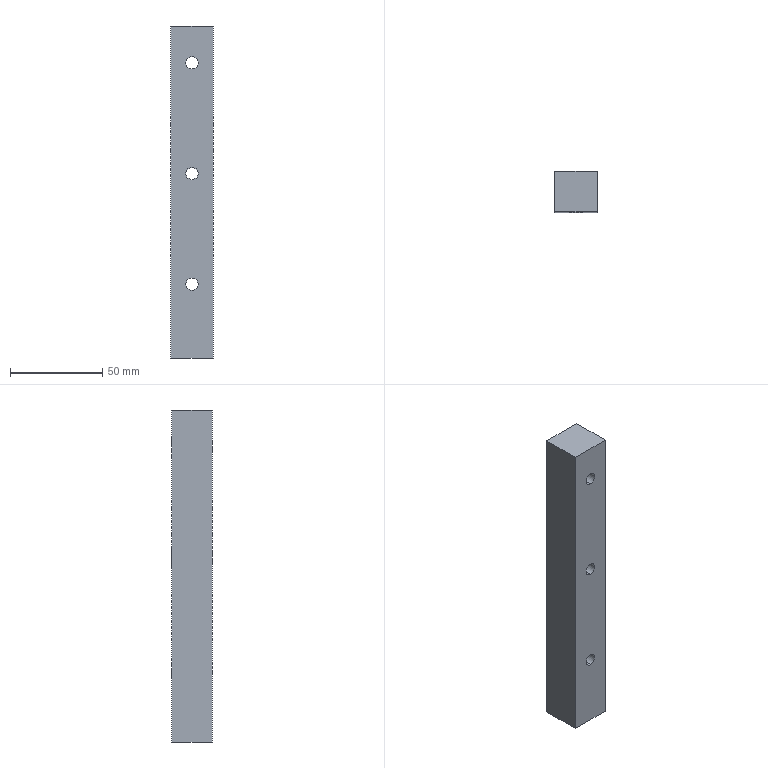Part | SolidWorks | features Extrusion 1, HoleWzd 1, LPattern 1 | 1 solid | 21 faces | box 23 x 22 x 180 mm | volume 87654 mm3 | cylinder 12 | plane 9 | commonest cylinder face diameters 6.6 x6 11 x6
STEP:
#1=CARTESIAN_POINT('',(11.5,15.6,34.5));
#2=VERTEX_POINT('',#1);
#3=CARTESIAN_POINT('',(11.5,15.6,45.5));
#4=VERTEX_POINT('',#3);
#5=CARTESIAN_POINT('',(11.5,15.6,40.));
#6=DIRECTION('',(0.,1.,0.));
#7=DIRECTION('',(0.,0.,1.));
#8=AXIS2_PLACEMENT_3D('',#5,#6,#7);
#9=CIRCLE('',#8,5.5);
#10=EDGE_CURVE('',#2,#4,#9,.T.);
#11=ORIENTED_EDGE('',*,*,#10,.F.);
#12=CARTESIAN_POINT('',(11.5,22.,34.5));
#13=VERTEX_POINT('',#12);
#14=CARTESIAN_POINT('',(11.5,22.,34.5));
#15=DIRECTION('',(0.,1.,0.));
#16=VECTOR('',#15,1000.);
#17=LINE('',#14,#16);
#18=EDGE_CURVE('',#2,#13,#17,.T.);
#19=ORIENTED_EDGE('',*,*,#18,.T.);
#20=CARTESIAN_POINT('',(11.5,22.,45.5));
#21=VERTEX_POINT('',#20);
#22=CARTESIAN_POINT('',(11.5,22.,40.));
#23=DIRECTION('',(0.,1.,0.));
#24=DIRECTION('',(0.,0.,1.));
#25=AXIS2_PLACEMENT_3D('',#22,#23,#24);
#26=CIRCLE('',#25,5.5);
#27=EDGE_CURVE('',#13,#21,#26,.T.);
#28=ORIENTED_EDGE('',*,*,#27,.T.);
#29=CARTESIAN_POINT('',(11.5,22.,45.5));
#30=DIRECTION('',(0.,1.,0.));
#31=VECTOR('',#30,1000.);
#32=LINE('',#29,#31);
#33=EDGE_CURVE('',#4,#21,#32,.T.);
#34=ORIENTED_EDGE('',*,*,#33,.F.);
#35=EDGE_LOOP('',(#11,#19,#28,#34));
#36=FACE_OUTER_BOUND('',#35,.T.);
#37=CARTESIAN_POINT('',(11.5,22.,40.));
#38=DIRECTION('',(0.,1.,0.));
#39=DIRECTION('',(0.,0.,1.));
#40=AXIS2_PLACEMENT_3D('',#37,#38,#39);
#41=CYLINDRICAL_SURFACE('',#40,5.5);
#42=ADVANCED_FACE('',(#36),#41,.F.);
#43=CARTESIAN_POINT('',(11.5,0.,36.7));
#44=VERTEX_POINT('',#43);
#45=CARTESIAN_POINT('',(11.5,0.,43.3));
#46=VERTEX_POINT('',#45);
#47=CARTESIAN_POINT('',(11.5,0.,40.));
#48=DIRECTION('',(0.,1.,0.));
#49=DIRECTION('',(0.,0.,1.));
#50=AXIS2_PLACEMENT_3D('',#47,#48,#49);
#51=CIRCLE('',#50,3.3);
#52=EDGE_CURVE('',#44,#46,#51,.T.);
#53=ORIENTED_EDGE('',*,*,#52,.F.);
#54=CARTESIAN_POINT('',(11.5,15.6,36.7));
#55=VERTEX_POINT('',#54);
#56=CARTESIAN_POINT('',(11.5,22.,36.7));
#57=DIRECTION('',(0.,1.,0.));
#58=VECTOR('',#57,1000.);
#59=LINE('',#56,#58);
#60=EDGE_CURVE('',#44,#55,#59,.T.);
#61=ORIENTED_EDGE('',*,*,#60,.T.);
#62=CARTESIAN_POINT('',(11.5,15.6,43.3));
#63=VERTEX_POINT('',#62);
#64=CARTESIAN_POINT('',(11.5,15.6,40.));
#65=DIRECTION('',(0.,1.,0.));
#66=DIRECTION('',(0.,0.,1.));
#67=AXIS2_PLACEMENT_3D('',#64,#65,#66);
#68=CIRCLE('',#67,3.3);
#69=EDGE_CURVE('',#55,#63,#68,.T.);
#70=ORIENTED_EDGE('',*,*,#69,.T.);
#71=CARTESIAN_POINT('',(11.5,22.,43.3));
#72=DIRECTION('',(0.,1.,0.));
#73=VECTOR('',#72,1000.);
#74=LINE('',#71,#73);
#75=EDGE_CURVE('',#46,#63,#74,.T.);
#76=ORIENTED_EDGE('',*,*,#75,.F.);
#77=EDGE_LOOP('',(#53,#61,#70,#76));
#78=FACE_OUTER_BOUND('',#77,.T.);
#79=CARTESIAN_POINT('',(11.5,22.,40.));
#80=DIRECTION('',(0.,1.,0.));
#81=DIRECTION('',(0.,0.,1.));
#82=AXIS2_PLACEMENT_3D('',#79,#80,#81);
#83=CYLINDRICAL_SURFACE('',#82,3.3);
#84=ADVANCED_FACE('',(#78),#83,.F.);
#85=CARTESIAN_POINT('',(11.5,15.6,94.5));
#86=VERTEX_POINT('',#85);
#87=CARTESIAN_POINT('',(11.5,15.6,105.5));
#88=VERTEX_POINT('',#87);
#89=CARTESIAN_POINT('',(11.5,15.6,100.));
#90=DIRECTION('',(0.,1.,0.));
#91=DIRECTION('',(0.,0.,1.));
#92=AXIS2_PLACEMENT_3D('',#89,#90,#91);
#93=CIRCLE('',#92,5.5);
#94=EDGE_CURVE('',#86,#88,#93,.T.);
#95=ORIENTED_EDGE('',*,*,#94,.F.);
#96=CARTESIAN_POINT('',(11.5,22.,94.5));
#97=VERTEX_POINT('',#96);
#98=CARTESIAN_POINT('',(11.5,22.,94.5));
#99=DIRECTION('',(0.,1.,0.));
#100=VECTOR('',#99,1000.);
#101=LINE('',#98,#100);
#102=EDGE_CURVE('',#86,#97,#101,.T.);
#103=ORIENTED_EDGE('',*,*,#102,.T.);
#104=CARTESIAN_POINT('',(11.5,22.,105.5));
#105=VERTEX_POINT('',#104);
#106=CARTESIAN_POINT('',(11.5,22.,100.));
#107=DIRECTION('',(0.,1.,0.));
#108=DIRECTION('',(0.,0.,1.));
#109=AXIS2_PLACEMENT_3D('',#106,#107,#108);
#110=CIRCLE('',#109,5.5);
#111=EDGE_CURVE('',#97,#105,#110,.T.);
#112=ORIENTED_EDGE('',*,*,#111,.T.);
#113=CARTESIAN_POINT('',(11.5,22.,105.5));
#114=DIRECTION('',(0.,1.,0.));
#115=VECTOR('',#114,1000.);
#116=LINE('',#113,#115);
#117=EDGE_CURVE('',#88,#105,#116,.T.);
#118=ORIENTED_EDGE('',*,*,#117,.F.);
#119=EDGE_LOOP('',(#95,#103,#112,#118));
#120=FACE_OUTER_BOUND('',#119,.T.);
#121=CARTESIAN_POINT('',(11.5,22.,100.));
#122=DIRECTION('',(0.,1.,0.));
#123=DIRECTION('',(0.,0.,1.));
#124=AXIS2_PLACEMENT_3D('',#121,#122,#123);
#125=CYLINDRICAL_SURFACE('',#124,5.5);
#126=ADVANCED_FACE('',(#120),#125,.F.);
#127=CARTESIAN_POINT('',(11.5,0.,96.7));
#128=VERTEX_POINT('',#127);
#129=CARTESIAN_POINT('',(11.5,0.,103.3));
#130=VERTEX_POINT('',#129);
#131=CARTESIAN_POINT('',(11.5,0.,100.));
#132=DIRECTION('',(0.,1.,0.));
#133=DIRECTION('',(0.,0.,1.));
#134=AXIS2_PLACEMENT_3D('',#131,#132,#133);
#135=CIRCLE('',#134,3.3);
#136=EDGE_CURVE('',#128,#130,#135,.T.);
#137=ORIENTED_EDGE('',*,*,#136,.F.);
#138=CARTESIAN_POINT('',(11.5,15.6,96.7));
#139=VERTEX_POINT('',#138);
#140=CARTESIAN_POINT('',(11.5,22.,96.7));
#141=DIRECTION('',(0.,1.,0.));
#142=VECTOR('',#141,1000.);
#143=LINE('',#140,#142);
#144=EDGE_CURVE('',#128,#139,#143,.T.);
#145=ORIENTED_EDGE('',*,*,#144,.T.);
#146=CARTESIAN_POINT('',(11.5,15.6,103.3));
#147=VERTEX_POINT('',#146);
#148=CARTESIAN_POINT('',(11.5,15.6,100.));
#149=DIRECTION('',(0.,1.,0.));
#150=DIRECTION('',(0.,0.,1.));
#151=AXIS2_PLACEMENT_3D('',#148,#149,#150);
#152=CIRCLE('',#151,3.3);
#153=EDGE_CURVE('',#139,#147,#152,.T.);
#154=ORIENTED_EDGE('',*,*,#153,.T.);
#155=CARTESIAN_POINT('',(11.5,22.,103.3));
#156=DIRECTION('',(0.,1.,0.));
#157=VECTOR('',#156,1000.);
#158=LINE('',#155,#157);
#159=EDGE_CURVE('',#130,#147,#158,.T.);
#160=ORIENTED_EDGE('',*,*,#159,.F.);
#161=EDGE_LOOP('',(#137,#145,#154,#160));
#162=FACE_OUTER_BOUND('',#161,.T.);
#163=CARTESIAN_POINT('',(11.5,22.,100.));
#164=DIRECTION('',(0.,1.,0.));
#165=DIRECTION('',(0.,0.,1.));
#166=AXIS2_PLACEMENT_3D('',#163,#164,#165);
#167=CYLINDRICAL_SURFACE('',#166,3.3);
#168=ADVANCED_FACE('',(#162),#167,.F.);
#169=CARTESIAN_POINT('',(11.5,15.6,154.5));
#170=VERTEX_POINT('',#169);
#171=CARTESIAN_POINT('',(11.5,15.6,165.5));
#172=VERTEX_POINT('',#171);
#173=CARTESIAN_POINT('',(11.5,15.6,160.));
#174=DIRECTION('',(0.,1.,0.));
#175=DIRECTION('',(0.,0.,1.));
#176=AXIS2_PLACEMENT_3D('',#173,#174,#175);
#177=CIRCLE('',#176,5.5);
#178=EDGE_CURVE('',#170,#172,#177,.T.);
#179=ORIENTED_EDGE('',*,*,#178,.F.);
#180=CARTESIAN_POINT('',(11.5,22.,154.5));
#181=VERTEX_POINT('',#180);
#182=CARTESIAN_POINT('',(11.5,22.,154.5));
#183=DIRECTION('',(0.,1.,0.));
#184=VECTOR('',#183,1000.);
#185=LINE('',#182,#184);
#186=EDGE_CURVE('',#170,#181,#185,.T.);
#187=ORIENTED_EDGE('',*,*,#186,.T.);
#188=CARTESIAN_POINT('',(11.5,22.,165.5));
#189=VERTEX_POINT('',#188);
#190=CARTESIAN_POINT('',(11.5,22.,160.));
#191=DIRECTION('',(0.,1.,0.));
#192=DIRECTION('',(0.,0.,1.));
#193=AXIS2_PLACEMENT_3D('',#190,#191,#192);
#194=CIRCLE('',#193,5.5);
#195=EDGE_CURVE('',#181,#189,#194,.T.);
#196=ORIENTED_EDGE('',*,*,#195,.T.);
#197=CARTESIAN_POINT('',(11.5,22.,165.5));
#198=DIRECTION('',(0.,1.,0.));
#199=VECTOR('',#198,1000.);
#200=LINE('',#197,#199);
#201=EDGE_CURVE('',#172,#189,#200,.T.);
#202=ORIENTED_EDGE('',*,*,#201,.F.);
#203=EDGE_LOOP('',(#179,#187,#196,#202));
#204=FACE_OUTER_BOUND('',#203,.T.);
#205=CARTESIAN_POINT('',(11.5,22.,160.));
#206=DIRECTION('',(0.,1.,0.));
#207=DIRECTION('',(0.,0.,1.));
#208=AXIS2_PLACEMENT_3D('',#205,#206,#207);
#209=CYLINDRICAL_SURFACE('',#208,5.5);
#210=ADVANCED_FACE('',(#204),#209,.F.);
#211=CARTESIAN_POINT('',(11.5,0.,156.7));
#212=VERTEX_POINT('',#211);
#213=CARTESIAN_POINT('',(11.5,0.,163.3));
#214=VERTEX_POINT('',#213);
#215=CARTESIAN_POINT('',(11.5,0.,160.));
#216=DIRECTION('',(0.,1.,0.));
#217=DIRECTION('',(0.,0.,1.));
#218=AXIS2_PLACEMENT_3D('',#215,#216,#217);
#219=CIRCLE('',#218,3.3);
#220=EDGE_CURVE('',#212,#214,#219,.T.);
#221=ORIENTED_EDGE('',*,*,#220,.F.);
#222=CARTESIAN_POINT('',(11.5,15.6,156.7));
#223=VERTEX_POINT('',#222);
#224=CARTESIAN_POINT('',(11.5,22.,156.7));
#225=DIRECTION('',(0.,1.,0.));
#226=VECTOR('',#225,1000.);
#227=LINE('',#224,#226);
#228=EDGE_CURVE('',#212,#223,#227,.T.);
#229=ORIENTED_EDGE('',*,*,#228,.T.);
#230=CARTESIAN_POINT('',(11.5,15.6,163.3));
#231=VERTEX_POINT('',#230);
#232=CARTESIAN_POINT('',(11.5,15.6,160.));
#233=DIRECTION('',(0.,1.,0.));
#234=DIRECTION('',(0.,0.,1.));
#235=AXIS2_PLACEMENT_3D('',#232,#233,#234);
#236=CIRCLE('',#235,3.3);
#237=EDGE_CURVE('',#223,#231,#236,.T.);
#238=ORIENTED_EDGE('',*,*,#237,.T.);
#239=CARTESIAN_POINT('',(11.5,22.,163.3));
#240=DIRECTION('',(0.,1.,0.));
#241=VECTOR('',#240,1000.);
#242=LINE('',#239,#241);
#243=EDGE_CURVE('',#214,#231,#242,.T.);
#244=ORIENTED_EDGE('',*,*,#243,.F.);
#245=EDGE_LOOP('',(#221,#229,#238,#244));
#246=FACE_OUTER_BOUND('',#245,.T.);
#247=CARTESIAN_POINT('',(11.5,22.,160.));
#248=DIRECTION('',(0.,1.,0.));
#249=DIRECTION('',(0.,0.,1.));
#250=AXIS2_PLACEMENT_3D('',#247,#248,#249);
#251=CYLINDRICAL_SURFACE('',#250,3.3);
#252=ADVANCED_FACE('',(#246),#251,.F.);
#253=CARTESIAN_POINT('',(0.,22.,0.));
#254=VERTEX_POINT('',#253);
#255=CARTESIAN_POINT('',(0.,0.,0.));
#256=VERTEX_POINT('',#255);
#257=CARTESIAN_POINT('',(0.,0.,0.));
#258=DIRECTION('',(0.,-1.,0.));
#259=VECTOR('',#258,1000.);
#260=LINE('',#257,#259);
#261=EDGE_CURVE('',#254,#256,#260,.T.);
#262=ORIENTED_EDGE('',*,*,#261,.T.);
#263=CARTESIAN_POINT('',(0.,0.,180.));
#264=VERTEX_POINT('',#263);
#265=CARTESIAN_POINT('',(0.,0.,180.));
#266=DIRECTION('',(0.,0.,-1.));
#267=VECTOR('',#266,1000.);
#268=LINE('',#265,#267);
#269=EDGE_CURVE('',#264,#256,#268,.T.);
#270=ORIENTED_EDGE('',*,*,#269,.F.);
#271=CARTESIAN_POINT('',(0.,22.,180.));
#272=VERTEX_POINT('',#271);
#273=CARTESIAN_POINT('',(0.,0.,180.));
#274=DIRECTION('',(0.,-1.,0.));
#275=VECTOR('',#274,1000.);
#276=LINE('',#273,#275);
#277=EDGE_CURVE('',#272,#264,#276,.T.);
#278=ORIENTED_EDGE('',*,*,#277,.F.);
#279=CARTESIAN_POINT('',(0.,22.,180.));
#280=DIRECTION('',(0.,0.,-1.));
#281=VECTOR('',#280,1000.);
#282=LINE('',#279,#281);
#283=EDGE_CURVE('',#272,#254,#282,.T.);
#284=ORIENTED_EDGE('',*,*,#283,.T.);
#285=EDGE_LOOP('',(#262,#270,#278,#284));
#286=FACE_OUTER_BOUND('',#285,.T.);
#287=CARTESIAN_POINT('',(0.,0.,180.));
#288=DIRECTION('',(1.,0.,0.));
#289=DIRECTION('',(0.,1.,0.));
#290=AXIS2_PLACEMENT_3D('',#287,#288,#289);
#291=PLANE('',#290);
#292=ADVANCED_FACE('',(#286),#291,.F.);
#293=CARTESIAN_POINT('',(11.5,0.,40.));
#294=DIRECTION('',(0.,1.,0.));
#295=DIRECTION('',(0.,0.,1.));
#296=AXIS2_PLACEMENT_3D('',#293,#294,#295);
#297=CIRCLE('',#296,3.3);
#298=EDGE_CURVE('',#46,#44,#297,.T.);
#299=ORIENTED_EDGE('',*,*,#298,.T.);
#300=ORIENTED_EDGE('',*,*,#52,.T.);
#301=EDGE_LOOP('',(#299,#300));
#302=FACE_BOUND('',#301,.T.);
#303=CARTESIAN_POINT('',(11.5,0.,100.));
#304=DIRECTION('',(0.,1.,0.));
#305=DIRECTION('',(0.,0.,1.));
#306=AXIS2_PLACEMENT_3D('',#303,#304,#305);
#307=CIRCLE('',#306,3.3);
#308=EDGE_CURVE('',#130,#128,#307,.T.);
#309=ORIENTED_EDGE('',*,*,#308,.T.);
#310=ORIENTED_EDGE('',*,*,#136,.T.);
#311=EDGE_LOOP('',(#309,#310));
#312=FACE_BOUND('',#311,.T.);
#313=CARTESIAN_POINT('',(11.5,0.,160.));
#314=DIRECTION('',(0.,1.,0.));
#315=DIRECTION('',(0.,0.,1.));
#316=AXIS2_PLACEMENT_3D('',#313,#314,#315);
#317=CIRCLE('',#316,3.3);
#318=EDGE_CURVE('',#214,#212,#317,.T.);
#319=ORIENTED_EDGE('',*,*,#318,.T.);
#320=ORIENTED_EDGE('',*,*,#220,.T.);
#321=EDGE_LOOP('',(#319,#320));
#322=FACE_BOUND('',#321,.T.);
#323=CARTESIAN_POINT('',(23.,0.,0.));
#324=VERTEX_POINT('',#323);
#325=CARTESIAN_POINT('',(0.,0.,0.));
#326=DIRECTION('',(1.,0.,0.));
#327=VECTOR('',#326,1000.);
#328=LINE('',#325,#327);
#329=EDGE_CURVE('',#256,#324,#328,.T.);
#330=ORIENTED_EDGE('',*,*,#329,.T.);
#331=CARTESIAN_POINT('',(23.,0.,180.));
#332=VERTEX_POINT('',#331);
#333=CARTESIAN_POINT('',(23.,0.,180.));
#334=DIRECTION('',(0.,0.,-1.));
#335=VECTOR('',#334,1000.);
#336=LINE('',#333,#335);
#337=EDGE_CURVE('',#332,#324,#336,.T.);
#338=ORIENTED_EDGE('',*,*,#337,.F.);
#339=CARTESIAN_POINT('',(0.,0.,180.));
#340=DIRECTION('',(1.,0.,0.));
#341=VECTOR('',#340,1000.);
#342=LINE('',#339,#341);
#343=EDGE_CURVE('',#264,#332,#342,.T.);
#344=ORIENTED_EDGE('',*,*,#343,.F.);
#345=ORIENTED_EDGE('',*,*,#269,.T.);
#346=EDGE_LOOP('',(#330,#338,#344,#345));
#347=FACE_OUTER_BOUND('',#346,.T.);
#348=CARTESIAN_POINT('',(0.,0.,180.));
#349=DIRECTION('',(0.,1.,0.));
#350=DIRECTION('',(0.,0.,1.));
#351=AXIS2_PLACEMENT_3D('',#348,#349,#350);
#352=PLANE('',#351);
#353=ADVANCED_FACE('',(#302,#312,#322,#347),#352,.F.);
#354=CARTESIAN_POINT('',(23.,22.,0.));
#355=VERTEX_POINT('',#354);
#356=CARTESIAN_POINT('',(23.,0.,0.));
#357=DIRECTION('',(0.,1.,0.));
#358=VECTOR('',#357,1000.);
#359=LINE('',#356,#358);
#360=EDGE_CURVE('',#324,#355,#359,.T.);
#361=ORIENTED_EDGE('',*,*,#360,.T.);
#362=CARTESIAN_POINT('',(23.,22.,180.));
#363=VERTEX_POINT('',#362);
#364=CARTESIAN_POINT('',(23.,22.,180.));
#365=DIRECTION('',(0.,0.,-1.));
#366=VECTOR('',#365,1000.);
#367=LINE('',#364,#366);
#368=EDGE_CURVE('',#363,#355,#367,.T.);
#369=ORIENTED_EDGE('',*,*,#368,.F.);
#370=CARTESIAN_POINT('',(23.,0.,180.));
#371=DIRECTION('',(0.,1.,0.));
#372=VECTOR('',#371,1000.);
#373=LINE('',#370,#372);
#374=EDGE_CURVE('',#332,#363,#373,.T.);
#375=ORIENTED_EDGE('',*,*,#374,.F.);
#376=ORIENTED_EDGE('',*,*,#337,.T.);
#377=EDGE_LOOP('',(#361,#369,#375,#376));
#378=FACE_OUTER_BOUND('',#377,.T.);
#379=CARTESIAN_POINT('',(23.,0.,180.));
#380=DIRECTION('',(-1.,0.,0.));
#381=DIRECTION('',(0.,-1.,0.));
#382=AXIS2_PLACEMENT_3D('',#379,#380,#381);
#383=PLANE('',#382);
#384=ADVANCED_FACE('',(#378),#383,.F.);
#385=CARTESIAN_POINT('',(11.5,22.,40.));
#386=DIRECTION('',(0.,1.,0.));
#387=DIRECTION('',(0.,0.,1.));
#388=AXIS2_PLACEMENT_3D('',#385,#386,#387);
#389=CIRCLE('',#388,5.5);
#390=EDGE_CURVE('',#21,#13,#389,.T.);
#391=ORIENTED_EDGE('',*,*,#390,.F.);
#392=ORIENTED_EDGE('',*,*,#27,.F.);
#393=EDGE_LOOP('',(#391,#392));
#394=FACE_BOUND('',#393,.T.);
#395=CARTESIAN_POINT('',(11.5,22.,100.));
#396=DIRECTION('',(0.,1.,0.));
#397=DIRECTION('',(0.,0.,1.));
#398=AXIS2_PLACEMENT_3D('',#395,#396,#397);
#399=CIRCLE('',#398,5.5);
#400=EDGE_CURVE('',#105,#97,#399,.T.);
#401=ORIENTED_EDGE('',*,*,#400,.F.);
#402=ORIENTED_EDGE('',*,*,#111,.F.);
#403=EDGE_LOOP('',(#401,#402));
#404=FACE_BOUND('',#403,.T.);
#405=CARTESIAN_POINT('',(11.5,22.,160.));
#406=DIRECTION('',(0.,1.,0.));
#407=DIRECTION('',(0.,0.,1.));
#408=AXIS2_PLACEMENT_3D('',#405,#406,#407);
#409=CIRCLE('',#408,5.5);
#410=EDGE_CURVE('',#189,#181,#409,.T.);
#411=ORIENTED_EDGE('',*,*,#410,.F.);
#412=ORIENTED_EDGE('',*,*,#195,.F.);
#413=EDGE_LOOP('',(#411,#412));
#414=FACE_BOUND('',#413,.T.);
#415=CARTESIAN_POINT('',(0.,22.,0.));
#416=DIRECTION('',(-1.,0.,0.));
#417=VECTOR('',#416,1000.);
#418=LINE('',#415,#417);
#419=EDGE_CURVE('',#355,#254,#418,.T.);
#420=ORIENTED_EDGE('',*,*,#419,.T.);
#421=ORIENTED_EDGE('',*,*,#283,.F.);
#422=CARTESIAN_POINT('',(0.,22.,180.));
#423=DIRECTION('',(-1.,0.,0.));
#424=VECTOR('',#423,1000.);
#425=LINE('',#422,#424);
#426=EDGE_CURVE('',#363,#272,#425,.T.);
#427=ORIENTED_EDGE('',*,*,#426,.F.);
#428=ORIENTED_EDGE('',*,*,#368,.T.);
#429=EDGE_LOOP('',(#420,#421,#427,#428));
#430=FACE_OUTER_BOUND('',#429,.T.);
#431=CARTESIAN_POINT('',(0.,22.,180.));
#432=DIRECTION('',(0.,-1.,0.));
#433=DIRECTION('',(0.,0.,-1.));
#434=AXIS2_PLACEMENT_3D('',#431,#432,#433);
#435=PLANE('',#434);
#436=ADVANCED_FACE('',(#394,#404,#414,#430),#435,.F.);
#437=ORIENTED_EDGE('',*,*,#277,.T.);
#438=ORIENTED_EDGE('',*,*,#343,.T.);
#439=ORIENTED_EDGE('',*,*,#374,.T.);
#440=ORIENTED_EDGE('',*,*,#426,.T.);
#441=EDGE_LOOP('',(#437,#438,#439,#440));
#442=FACE_OUTER_BOUND('',#441,.T.);
#443=CARTESIAN_POINT('',(0.,0.,180.));
#444=DIRECTION('',(0.,0.,-1.));
#445=DIRECTION('',(-1.,0.,0.));
#446=AXIS2_PLACEMENT_3D('',#443,#444,#445);
#447=PLANE('',#446);
#448=ADVANCED_FACE('',(#442),#447,.F.);
#449=ORIENTED_EDGE('',*,*,#261,.F.);
#450=ORIENTED_EDGE('',*,*,#419,.F.);
#451=ORIENTED_EDGE('',*,*,#360,.F.);
#452=ORIENTED_EDGE('',*,*,#329,.F.);
#453=EDGE_LOOP('',(#449,#450,#451,#452));
#454=FACE_OUTER_BOUND('',#453,.T.);
#455=CARTESIAN_POINT('',(0.,0.,0.));
#456=DIRECTION('',(0.,0.,-1.));
#457=DIRECTION('',(-1.,0.,0.));
#458=AXIS2_PLACEMENT_3D('',#455,#456,#457);
#459=PLANE('',#458);
#460=ADVANCED_FACE('',(#454),#459,.T.);
#461=ORIENTED_EDGE('',*,*,#228,.F.);
#462=ORIENTED_EDGE('',*,*,#318,.F.);
#463=ORIENTED_EDGE('',*,*,#243,.T.);
#464=CARTESIAN_POINT('',(11.5,15.6,160.));
#465=DIRECTION('',(0.,1.,0.));
#466=DIRECTION('',(0.,0.,1.));
#467=AXIS2_PLACEMENT_3D('',#464,#465,#466);
#468=CIRCLE('',#467,3.3);
#469=EDGE_CURVE('',#231,#223,#468,.T.);
#470=ORIENTED_EDGE('',*,*,#469,.T.);
#471=EDGE_LOOP('',(#461,#462,#463,#470));
#472=FACE_OUTER_BOUND('',#471,.T.);
#473=CARTESIAN_POINT('',(11.5,22.,160.));
#474=DIRECTION('',(0.,1.,0.));
#475=DIRECTION('',(0.,0.,1.));
#476=AXIS2_PLACEMENT_3D('',#473,#474,#475);
#477=CYLINDRICAL_SURFACE('',#476,3.3);
#478=ADVANCED_FACE('',(#472),#477,.F.);
#479=ORIENTED_EDGE('',*,*,#469,.F.);
#480=ORIENTED_EDGE('',*,*,#237,.F.);
#481=EDGE_LOOP('',(#479,#480));
#482=FACE_BOUND('',#481,.T.);
#483=CARTESIAN_POINT('',(11.5,15.6,160.));
#484=DIRECTION('',(0.,1.,0.));
#485=DIRECTION('',(0.,0.,1.));
#486=AXIS2_PLACEMENT_3D('',#483,#484,#485);
#487=CIRCLE('',#486,5.5);
#488=EDGE_CURVE('',#172,#170,#487,.T.);
#489=ORIENTED_EDGE('',*,*,#488,.T.);
#490=ORIENTED_EDGE('',*,*,#178,.T.);
#491=EDGE_LOOP('',(#489,#490));
#492=FACE_OUTER_BOUND('',#491,.T.);
#493=CARTESIAN_POINT('',(14.8,15.6,160.));
#494=DIRECTION('',(0.,-1.,0.));
#495=DIRECTION('',(0.,0.,-1.));
#496=AXIS2_PLACEMENT_3D('',#493,#494,#495);
#497=PLANE('',#496);
#498=ADVANCED_FACE('',(#482,#492),#497,.F.);
#499=ORIENTED_EDGE('',*,*,#186,.F.);
#500=ORIENTED_EDGE('',*,*,#488,.F.);
#501=ORIENTED_EDGE('',*,*,#201,.T.);
#502=ORIENTED_EDGE('',*,*,#410,.T.);
#503=EDGE_LOOP('',(#499,#500,#501,#502));
#504=FACE_OUTER_BOUND('',#503,.T.);
#505=CARTESIAN_POINT('',(11.5,22.,160.));
#506=DIRECTION('',(0.,1.,0.));
#507=DIRECTION('',(0.,0.,1.));
#508=AXIS2_PLACEMENT_3D('',#505,#506,#507);
#509=CYLINDRICAL_SURFACE('',#508,5.5);
#510=ADVANCED_FACE('',(#504),#509,.F.);
#511=ORIENTED_EDGE('',*,*,#144,.F.);
#512=ORIENTED_EDGE('',*,*,#308,.F.);
#513=ORIENTED_EDGE('',*,*,#159,.T.);
#514=CARTESIAN_POINT('',(11.5,15.6,100.));
#515=DIRECTION('',(0.,1.,0.));
#516=DIRECTION('',(0.,0.,1.));
#517=AXIS2_PLACEMENT_3D('',#514,#515,#516);
#518=CIRCLE('',#517,3.3);
#519=EDGE_CURVE('',#147,#139,#518,.T.);
#520=ORIENTED_EDGE('',*,*,#519,.T.);
#521=EDGE_LOOP('',(#511,#512,#513,#520));
#522=FACE_OUTER_BOUND('',#521,.T.);
#523=CARTESIAN_POINT('',(11.5,22.,100.));
#524=DIRECTION('',(0.,1.,0.));
#525=DIRECTION('',(0.,0.,1.));
#526=AXIS2_PLACEMENT_3D('',#523,#524,#525);
#527=CYLINDRICAL_SURFACE('',#526,3.3);
#528=ADVANCED_FACE('',(#522),#527,.F.);
#529=ORIENTED_EDGE('',*,*,#519,.F.);
#530=ORIENTED_EDGE('',*,*,#153,.F.);
#531=EDGE_LOOP('',(#529,#530));
#532=FACE_BOUND('',#531,.T.);
#533=CARTESIAN_POINT('',(11.5,15.6,100.));
#534=DIRECTION('',(0.,1.,0.));
#535=DIRECTION('',(0.,0.,1.));
#536=AXIS2_PLACEMENT_3D('',#533,#534,#535);
#537=CIRCLE('',#536,5.5);
#538=EDGE_CURVE('',#88,#86,#537,.T.);
#539=ORIENTED_EDGE('',*,*,#538,.T.);
#540=ORIENTED_EDGE('',*,*,#94,.T.);
#541=EDGE_LOOP('',(#539,#540));
#542=FACE_OUTER_BOUND('',#541,.T.);
#543=CARTESIAN_POINT('',(14.8,15.6,100.));
#544=DIRECTION('',(0.,-1.,0.));
#545=DIRECTION('',(0.,0.,-1.));
#546=AXIS2_PLACEMENT_3D('',#543,#544,#545);
#547=PLANE('',#546);
#548=ADVANCED_FACE('',(#532,#542),#547,.F.);
#549=ORIENTED_EDGE('',*,*,#102,.F.);
#550=ORIENTED_EDGE('',*,*,#538,.F.);
#551=ORIENTED_EDGE('',*,*,#117,.T.);
#552=ORIENTED_EDGE('',*,*,#400,.T.);
#553=EDGE_LOOP('',(#549,#550,#551,#552));
#554=FACE_OUTER_BOUND('',#553,.T.);
#555=CARTESIAN_POINT('',(11.5,22.,100.));
#556=DIRECTION('',(0.,1.,0.));
#557=DIRECTION('',(0.,0.,1.));
#558=AXIS2_PLACEMENT_3D('',#555,#556,#557);
#559=CYLINDRICAL_SURFACE('',#558,5.5);
#560=ADVANCED_FACE('',(#554),#559,.F.);
#561=ORIENTED_EDGE('',*,*,#60,.F.);
#562=ORIENTED_EDGE('',*,*,#298,.F.);
#563=ORIENTED_EDGE('',*,*,#75,.T.);
#564=CARTESIAN_POINT('',(11.5,15.6,40.));
#565=DIRECTION('',(0.,1.,0.));
#566=DIRECTION('',(0.,0.,1.));
#567=AXIS2_PLACEMENT_3D('',#564,#565,#566);
#568=CIRCLE('',#567,3.3);
#569=EDGE_CURVE('',#63,#55,#568,.T.);
#570=ORIENTED_EDGE('',*,*,#569,.T.);
#571=EDGE_LOOP('',(#561,#562,#563,#570));
#572=FACE_OUTER_BOUND('',#571,.T.);
#573=CARTESIAN_POINT('',(11.5,22.,40.));
#574=DIRECTION('',(0.,1.,0.));
#575=DIRECTION('',(0.,0.,1.));
#576=AXIS2_PLACEMENT_3D('',#573,#574,#575);
#577=CYLINDRICAL_SURFACE('',#576,3.3);
#578=ADVANCED_FACE('',(#572),#577,.F.);
#579=ORIENTED_EDGE('',*,*,#569,.F.);
#580=ORIENTED_EDGE('',*,*,#69,.F.);
#581=EDGE_LOOP('',(#579,#580));
#582=FACE_BOUND('',#581,.T.);
#583=CARTESIAN_POINT('',(11.5,15.6,40.));
#584=DIRECTION('',(0.,1.,0.));
#585=DIRECTION('',(0.,0.,1.));
#586=AXIS2_PLACEMENT_3D('',#583,#584,#585);
#587=CIRCLE('',#586,5.5);
#588=EDGE_CURVE('',#4,#2,#587,.T.);
#589=ORIENTED_EDGE('',*,*,#588,.T.);
#590=ORIENTED_EDGE('',*,*,#10,.T.);
#591=EDGE_LOOP('',(#589,#590));
#592=FACE_OUTER_BOUND('',#591,.T.);
#593=CARTESIAN_POINT('',(14.8,15.6,40.));
#594=DIRECTION('',(0.,-1.,0.));
#595=DIRECTION('',(0.,0.,-1.));
#596=AXIS2_PLACEMENT_3D('',#593,#594,#595);
#597=PLANE('',#596);
#598=ADVANCED_FACE('',(#582,#592),#597,.F.);
#599=ORIENTED_EDGE('',*,*,#18,.F.);
#600=ORIENTED_EDGE('',*,*,#588,.F.);
#601=ORIENTED_EDGE('',*,*,#33,.T.);
#602=ORIENTED_EDGE('',*,*,#390,.T.);
#603=EDGE_LOOP('',(#599,#600,#601,#602));
#604=FACE_OUTER_BOUND('',#603,.T.);
#605=CARTESIAN_POINT('',(11.5,22.,40.));
#606=DIRECTION('',(0.,1.,0.));
#607=DIRECTION('',(0.,0.,1.));
#608=AXIS2_PLACEMENT_3D('',#605,#606,#607);
#609=CYLINDRICAL_SURFACE('',#608,5.5);
#610=ADVANCED_FACE('',(#604),#609,.F.);
#611=CLOSED_SHELL('',(#42,#84,#126,#168,#210,#252,#292,#353,#384,#436,#448,#460,#478,#498,#510,#528,#548,#560,#578,#598,#610));
#612=MANIFOLD_SOLID_BREP('',#611);
#613=CARTESIAN_POINT('',(0.,0.,0.));
#614=DIRECTION('',(0.,0.,1.));
#615=DIRECTION('',(1.,0.,0.));
#616=AXIS2_PLACEMENT_3D('',#613,#614,#615);
#617=(LENGTH_UNIT()NAMED_UNIT(*)SI_UNIT(.MILLI.,.METRE.));
#618=UNCERTAINTY_MEASURE_WITH_UNIT(LENGTH_MEASURE(0.00001),#617,'','');
#619=(NAMED_UNIT(*)PLANE_ANGLE_UNIT()SI_UNIT($,.RADIAN.));
#620=(NAMED_UNIT(*)SI_UNIT($,.STERADIAN.)SOLID_ANGLE_UNIT());
#621=(GEOMETRIC_REPRESENTATION_CONTEXT(3)GLOBAL_UNCERTAINTY_ASSIGNED_CONTEXT((#618))GLOBAL_UNIT_ASSIGNED_CONTEXT((#617,#619,#620))REPRESENTATION_CONTEXT('',''));
#622=ADVANCED_BREP_SHAPE_REPRESENTATION('',(#612,#616),#621);